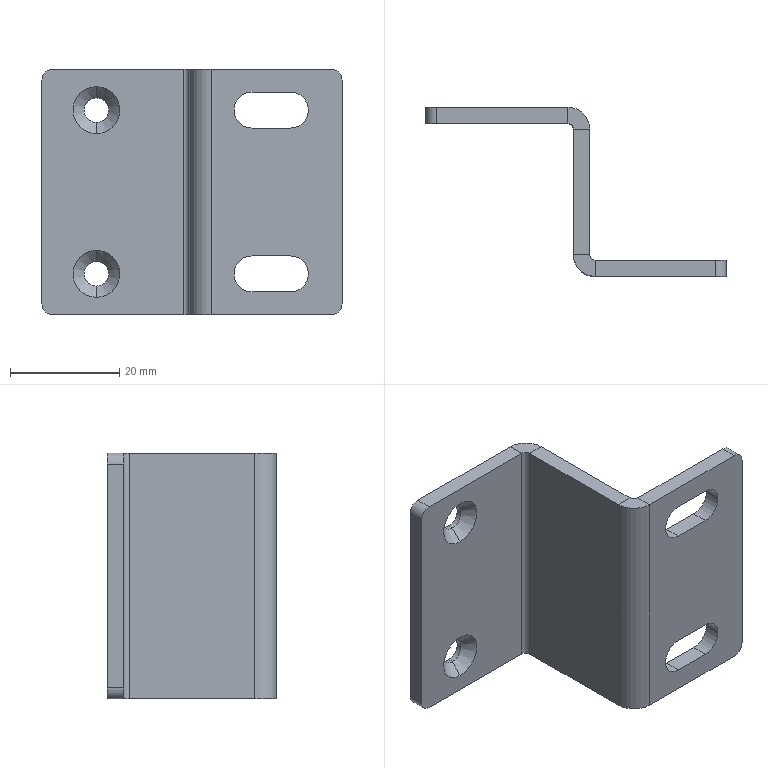Part | STEP file | Tabletop mounting plate B | 1 solid | 42 faces | box 55 x 31 x 45 mm | volume 10250 mm3 | plane 22 | cylinder 16 | cone 4 | commonest cylinder face diameters 4 x4 4.5 x4 6.6 x4 2 x2 8 x2